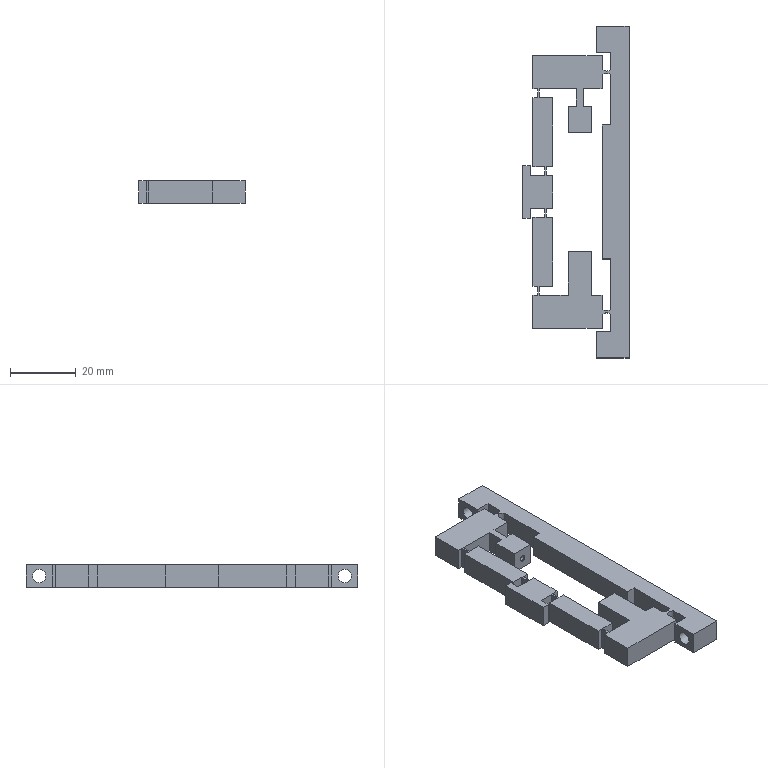Part | NX | features DATUM_CSYS 5, SKETCH 5, EXTRUDE 4, EXTRACT_FACE 2, BREP 1, CHAMFER 1, HOLE PACKAGE 1, Instance Feature 1, Mirror Feature 1, OFFSET_REGION 1, SIMPLE HOLE 1 | 1 solid | 81 faces | box 32.2 x 100.6 x 6.8 mm | volume 11129 mm3 | plane 70 | cylinder 9 | cone 2 | commonest cylinder face diameters 3.356 x3 3.36 x3 4 x2 1.5 x1